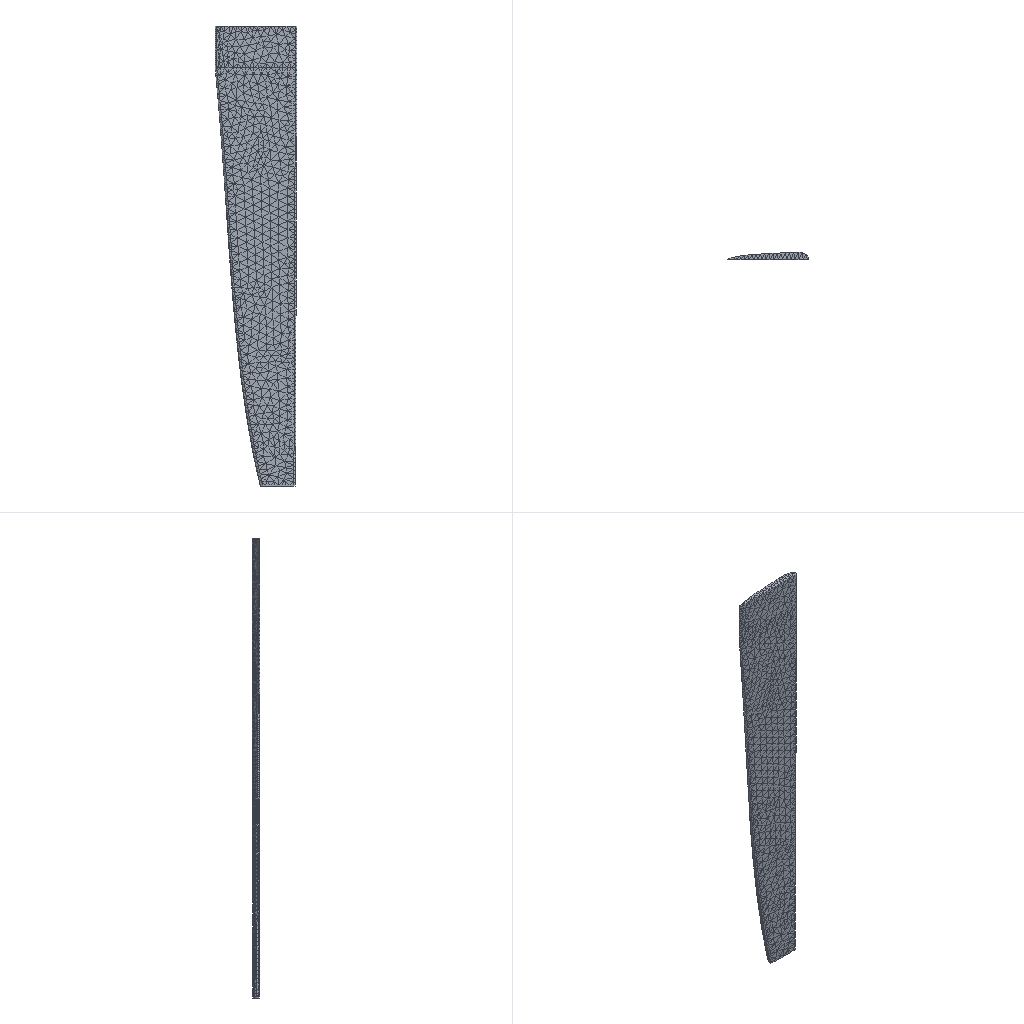Simulation study | ansys workbench
Set-up summary:
category,name,step,type,value,unit,region
solver,ansys_workbench
units,mm-N-s-tonne (MPa),,stated,"/units,MPA"
analysis,LS1,,static
load_step,LS1,LS1,static,nsubst=1; time=1
mesh,nodes,,,10822
mesh,elements,,,7060
element_type,SOLID187,,,5148
element_type,SURF154,,,1912
material,Structural Steel,,E,200000,tonne s^-2 mm^-1
material,Structural Steel,,nu,0.3
material,Structural Steel,,density,7.85e-09,tonne mm^-3
material,Structural Steel,,conductivity,60.5,tonne mm s^-3 C^-1
material,Structural Steel,,specific_heat,4.34e+08,mm^2 s^-2 C^-1
material,Structural Steel,,cte,1.2e-05,C^-1
material,Structural Steel,,permeability,10000
material,Structural Steel,,resistivity,0.00017,ohm mm
load,Define Force Using Surface Effect Elements,LS1,surface-effect pres face 1,0.0007902,,SURF154 #2
bc,Fixed Supports,model,fixed,[dofs=ALL],,_FIXEDSU
named_set,_FIXEDSU,,node,135
Ansys APDL input file, long lists of numbers shortened:
/batch
/config,noeldb,1     ! force off writing results to database
*get,_wallstrt,active,,time,wall
! ANSYS input file written by Workbench version 2022 R1
! File used for geometry attach:
/title,1111--____ (B5)
! ****** Begin Custom Load Command Snippet ******
/COM, ACT Extensions:
/COM,     LSDYNA, 2021.1
/COM,
! ****** End   Custom Load Command Snippet ******
*DIM,_wb_ProjectScratch_dir,string,248
_wb_ProjectScratch_dir(1) = ''
*DIM,_wb_SolverFiles_dir,string,248
_wb_SolverFiles_dir(1) = ''
*DIM,_wb_userfiles_dir,string,248
_wb_userfiles_dir(1) = ''
/com,--- Data in consistent NMM units. See Solving Units in the help system for more information.
/units,MPA
/nopr
/wb,file,start              !  signify a WB generated input file
/prep7
! Turn off shape checking because checks already performed inside WB mesher.
! See help system for more information.
SHPP,OFF,,NOWARN
/nolist
etcon,set             ! allow ANSYS to choose best KEYOP's for 180x elements, resets any applicable keyopt to MAPDL defaults
/com,*********** Nodes for the whole assembly ***********
nblock,3,,11904
(1i9,3e20.9e3)
        1     5.822691343E+03     8.726655121E+01    -5.000000000E+04
! (10821 more lines like these left out)
-1
/wb,elem,start            !  set before creation of elements
/com,*********** Elements for Body 1 "__1111-FreeParts|NONE" ***********
et,1,187
eblock,19,solid,,5148
(19i9)
        1        1        1        1        0        0        0        0       10        0        1      529     1736     1913     1886     5205    10583     5207     5206
! (10295 more lines like these left out)
-1
/wb,elem,end               !  done creating elements
/com,*********** Send User Defined Coordinate System(s) ***********
csys,0
toffst,273.15,  ! Temperature offset from absolute zero
/com,*********** Set Reference Temperature ***********
tref,22.
/wb,mat,start              !  starting to send materials
/com,*********** Send Materials ***********
Temperature = 'TEMP' ! Temperature
MP,DENS,1,7.85e-09,	! tonne mm^-3
MP,ALPX,1,1.2e-05,	! C^-1
MP,C,1,434000000,	! mm^2 s^-2 C^-1
MP,KXX,1,60.5,	! tonne mm s^-3 C^-1
MP,RSVX,1,0.00017,	! ohm mm
MP,EX,1,200000,	! tonne s^-2 mm^-1
MP,NUXY,1,0.3,
MP,MURX,1,10000,
/wb,mat,end                !  done sending materials
!************************* Model Summary ********************
!__1111-FreeParts|NONE,	结构钢,	matid,	1
!************************* End Model Summary ********************
! get the diagonal of the bounding box. Needed later for other things
*get,_xmin,node,,mnloc,x
*get,_ymin,node,,mnloc,y
*get,_zmin,node,,mnloc,z
*get,_xmax,node,,mxloc,x
*get,_ymax,node,,mxloc,y
*get,_zmax,node,,mxloc,z
_ASMDIAG=(_xmax-_xmin)*(_xmax-_xmin)+(_ymax-_ymin)*(_ymax-_ymin)+(_zmax-_zmin)*(_zmax-_zmin)
_ASMDIAG=SQRT(_ASMDIAG)
/wb,contact,start          !  starting to send contact
/wb,contact,end            !  done creating contacts
/golist
/wb,load,start             !  starting to send loads
/com,*********** Fixed Supports ***********
CMBLOCK,_FIXEDSU,NODE,      135
(8i10)
       567       577       578       579       580       581       582       583
! (16 more lines like these left out)
cmsel,s,_FIXEDSU
d,all,all
nsel,all
/com,*********** Define Force Using Surface Effect Elements ***********
local,12,0,0.,0.,0.,0.,0.,0.
csys,0
et,2,154
eblock,10,,,1912
(15i9)
     8843        2        2        2       12      848      962     1040     1040     6540     7569     1040     6543
! (1911 more lines like these left out)
-1
esel,s,type,,2
keyop,2,2,1                ! Apply load in local coordinate system
keyop,2,7,1                ! Use original area so load is constant in large deformation
esel,all
/gst,on,on
fini
*get,_numnode,node,0,count
*get,_numelem,elem,0,count
*get, _MAXELEMNUM, elem, 0, NUM, MAX
*get, _MAXNODENUM, node, 0, NUM, MAX
*get, _MAXELEMTYPE, etyp, 0, NUM, MAX
*get, _MAXREALCONST, real, 0, NUM, MAX
/go
/wb,load,end               !  done creating loads
/com,--- Number of total nodes = %_numnode%
/com,--- Number of contact elements = 1912
/com,--- Number of spring elements = 0
/com,--- Number of bearing elements = 0
/com,--- Number of solid elements = 5148
/com,--- Number of condensed parts = 0
/com,--- Number of total elements = %_numelem%
*get,_wallbsol,active,,time,wall
/com,****************************************************************************
/com,*************************    SOLUTION       ********************************
/com,****************************************************************************
/solu
antype,0                   ! static analysis
_thickRatio=  0     ! Ratio of thick parts in the model
eqsl,sparse,,,,,1
cntr,print,1               ! print out contact info and also make no initial contact an error
dmpoption,emat,no             ! Don't combine emat file for DANSYS
dmpoption,esav,no             ! Don't combine esav file for DANSYS
nldiag,cont,iter           ! print out contact info each equilibrium iteration
rescontrol,,none                 ! Do not keep any restart files
/com,****************************************************
/com,******************* SOLVE FOR LS 1 OF 1 ****************
esel,s,type,,2
nsle
sfe,all,1,pres,1,7.90197778072358e-004
sfe,all,2,pres,1,0.
sfe,all,3,pres,1,0.
nsel,all
esel,all
/nopr
/gopr
nsub,1,1,1
time,1.
outres,erase
outres,all,none
outres,nsol,all,
outres,rsol,all
outres,eangl,all
outres,etmp,all
outres,veng,all
outres,strs,all,
outres,epel,all,
outres,eppl,all,
outres,cont,all,
! *********** WB SOLVE COMMAND ***********
! check interactive state
*get,ANSINTER_,active,,int
*if,ANSINTER_,ne,0,then
/eof
*endif
solve
/com *************** Write FE CONNECTORS *********
CEWRITE,file,ce,,INTE
/com,****************************************************
/com,*************** FINISHED SOLVE FOR LS 1 *************
*get,_wallasol,active,,time,wall
/nopr
*get,_numnode,node,0,count
*get,_numelem,elem,0,count
*get, _MAXELEMNUM, elem, 0, NUM, MAX
*get, _MAXNODENUM, node, 0, NUM, MAX,,,INTERNAL
*get, _MAXELEMTYPE, etyp, 0, NUM, MAX
*get, _MAXREALCONST, real, 0, NUM, MAX
/gopr
/post1
xmlo,ENCODING,ISO-8859-1
xmlo,parm
/xml,parm,xml
fini
/gopr
*get,_walldone,active,,time,wall
_preptime=(_wallbsol-_wallstrt)*3600
_solvtime=(_wallasol-_wallbsol)*3600
_posttime=(_walldone-_wallasol)*3600
_totaltim=(_walldone-_wallstrt)*3600
*get,_dlbratio,active,0,solu,dlbr
*get,_combtime,active,0,solu,comb
*get,_ssmode,active,0,solu,ssmm
*get,_ndofs,active,0,solu,ndof
*get,_sol_end_time,active,0,set,time
*if,_sol_end_time,eq,1.,then
/fclean				!clean distributed files
*endif
/com,--- Total number of nodes = %_numnode%
/com,--- Total number of elements = %_numelem%
/com,--- Element load balance ratio = %_dlbratio%
/com,--- Time to combine distributed files = %_combtime%
/com,--- Sparse memory mode = %_ssmode%
/com,--- Number of DOF = %_ndofs%
/wb,file,end               ! done with WB generated input
Results summary:
result,analyses[0].index,,,1
result,analyses[0].system,,,SYS
result,analyses[0].deck,,,deck.dat
result,analyses[0].solve_status,,,completed
result,analyses[0].analysis_type,,,static
result,analyses[0].physics,,,mechanical
result,analyses[0].unit_system,,,"NMM: mm, ton, N, s, mV, mA, degC"
result,analyses[0].n_sets,,,1
result,analyses[0].load_steps[0].set,set=1,,1
result,analyses[0].load_steps[0].time_or_freq,set=1,,1
result,analyses[0].load_steps[0].max_displacement_magnitude,set=1,,2.82
result,analyses[0].load_steps[0].max_von_mises_nodal,set=1,,2.802
result,analyses[0].load_steps[0].reaction_force_sum_xyz[1],set=1,,-361990
result,analyses[0].load_steps[0].reaction_force_sum_xyz[2],set=1,,9.17045e-07
result,analyses[0].load_steps[0].reaction_force_sum_xyz[3],set=1,,-2.50632e-06